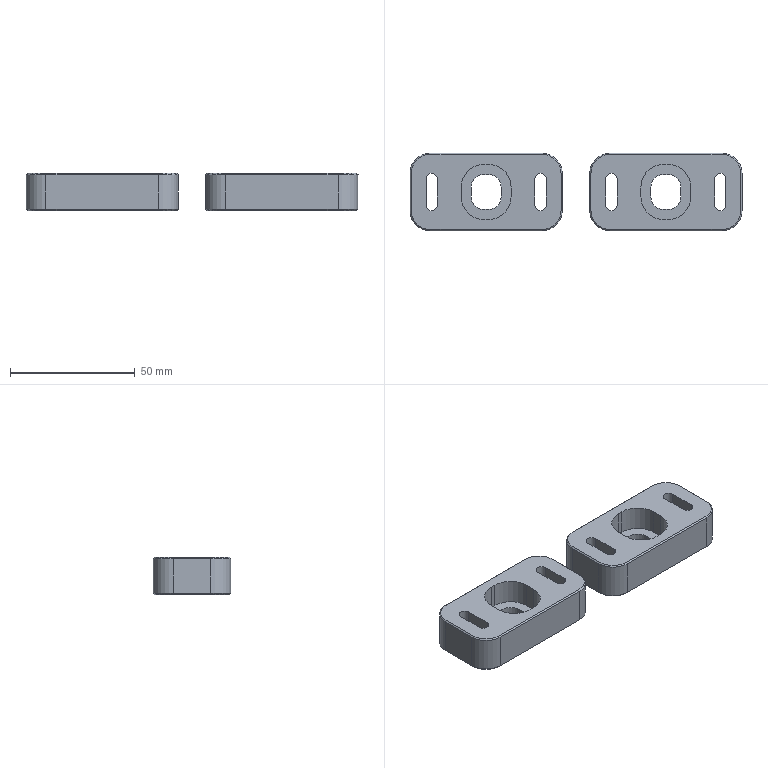NC program | NX | posted with a generic post | part box 133 x 31 x 15 mm
Whole program:
N10 G17 G21 G94 G90
(ZLEVEL_PROFILE_1_COPY_1_COPY_COPY , TOOL : D4A45)
N12 T02 M6
N14 G54
N16 G17 G0 G90 X58.268 Y-5.399 S9500 M3
N18 G43 Z30. H2
N20 Z0.
N22 G94 G1 Z-1. F1000.
N24 X58.891 Y-5.596
N26 G3 X59.091 Y-5.25 R0.4
N28 G1 Y5.25
N30 G3 X57.8 Y6.541 R1.291
N32 X56.509 Y5.25 R1.291
N34 G1 Y-5.25
N36 G3 X57.8 Y-6.541 R1.291
N38 X59.091 Y-5.25 R1.291
N40 X58.891 Y-4.904 R0.4
N42 G1 X58.291 Y-4.557
N44 Z0.
N46 G0 Z30.
N48 X14.668 Y-5.399
N50 Z0.
N52 G1 Z-1.
N54 X15.291 Y-5.596
N56 G3 X15.491 Y-5.25 R0.4
N58 G1 Y5.25
N60 G3 X14.2 Y6.541 R1.291
N62 X12.909 Y5.25 R1.291
N64 G1 Y-5.25
N66 G3 X14.2 Y-6.541 R1.291
N68 X15.491 Y-5.25 R1.291
N70 X15.291 Y-4.904 R0.4
N72 G1 X14.691 Y-4.557
N74 Z0.
N76 G0 Z30.
N78 X34.257 Y-5.155
N80 Z0.
N82 G1 Z-1.
N84 X34.654 Y-5.841
N86 G3 X35. Y-6.041 R0.4
N88 G1 X37.
N90 G3 X41.041 Y-2. R4.041
N92 G1 Y2.
N94 G3 X37. Y6.041 R4.041
N96 G1 X35.
N98 G3 X30.959 Y2. R4.041
N100 G1 Y-2.
N102 G3 X35. Y-6.041 R4.041
N104 X35.346 Y-5.841 R0.4
N106 G1 X35.693 Y-5.241
N108 Z0.
N110 G0 Z30.
N112 X-58.268 Y5.399
N114 Z0.
N116 G1 Z-1.
N118 X-58.891 Y5.596
N120 G3 X-59.091 Y5.25 R0.4
N122 G1 Y-5.25
N124 G3 X-57.8 Y-6.541 R1.291
N126 X-56.509 Y-5.25 R1.291
N128 G1 Y5.25
N130 G3 X-57.8 Y6.541 R1.291
N132 X-59.091 Y5.25 R1.291
N134 X-58.891 Y4.904 R0.4
N136 G1 X-58.291 Y4.557
N138 Z0.
N140 G0 Z30.
N142 X-34.257 Y5.155
N144 Z0.
N146 G1 Z-1.
N148 X-34.654 Y5.841
N150 G3 X-35. Y6.041 R0.4
N152 G1 X-37.
N154 G3 X-41.041 Y2. R4.041
N156 G1 Y-2.
N158 G3 X-37. Y-6.041 R4.041
N160 G1 X-35.
N162 G3 X-30.959 Y-2. R4.041
N164 G1 Y2.
N166 G3 X-35. Y6.041 R4.041
N168 X-35.346 Y5.841 R0.4
N170 G1 X-35.693 Y5.241
N172 Z0.
N174 G0 Z30.
N176 X-14.668 Y5.399
N178 Z0.
N180 G1 Z-1.
N182 X-15.291 Y5.596
N184 G3 X-15.491 Y5.25 R0.4
N186 G1 Y-5.25
N188 G3 X-14.2 Y-6.541 R1.291
N190 X-12.909 Y-5.25 R1.291
N192 G1 Y5.25
N194 G3 X-14.2 Y6.541 R1.291
N196 X-15.491 Y5.25 R1.291
N198 X-15.291 Y4.904 R0.4
N200 G1 X-14.691 Y4.557
N202 Z0.
N204 G0 Z30.
N206 X-59.175 Y16.734
N208 Z0.
N210 G1 Z-1.
N212 X-58.843 Y16.159
N214 G3 X-58.497 Y15.959 R0.4
N216 G1 X-13.5
N218 G2 X-5.041 Y7.503 R8.459
N220 G1 Y-7.5
N222 G2 X-13.499 Y-15.959 R8.459
N224 G1 X-58.5
N226 G2 X-66.959 Y-7.503 R8.459
N228 G1 Y7.5
N230 G2 X-58.497 Y15.959 R8.459
N232 G3 X-58.15 Y16.158 R0.4
N234 G1 X-57.804 Y16.759
N236 Z0.
N238 G0 Z30.
N240 X12.821 Y16.734
N242 Z0.
N244 G1 Z-1.
N246 X13.153 Y16.159
N248 G3 X13.499 Y15.959 R0.4
N250 G1 X58.5
N252 G2 X66.959 Y7.503 R8.459
N254 G1 Y-7.5
N256 G2 X58.497 Y-15.959 R8.459
N258 G1 X13.5
N260 G2 X5.041 Y-7.503 R8.459
N262 G1 Y7.5
N264 G2 X13.499 Y15.959 R8.459
N266 G3 X13.846 Y16.159 R0.4
N268 G1 X14.192 Y16.759
N270 Z0.
N272 G0 Z30.
N274 M5
N276 M2